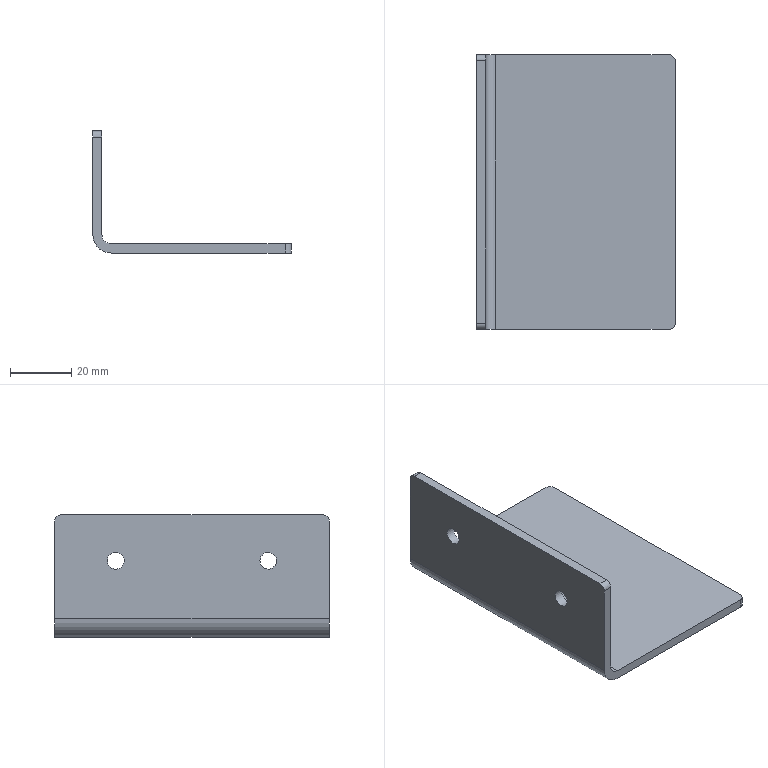Part | NX | features 5003_229_Bracket 2 | 1 solid | 16 faces | box 65 x 90 x 40 mm | volume 26866 mm3 | plane 8 | cylinder 8 | commonest cylinder face diameters 4 x4 5.5 x2 6 x1 12 x1
STEP:
#1=CARTESIAN_POINT('',(218.525,-127.,-84.75));
#2=VERTEX_POINT('',#1);
#3=CARTESIAN_POINT('',(218.525,-127.,-82.));
#4=DIRECTION('',(1.,0.,0.));
#5=DIRECTION('',(0.,0.,-1.));
#6=AXIS2_PLACEMENT_3D('',#3,#4,#5);
#7=CIRCLE('',#6,2.75);
#8=EDGE_CURVE('',#2,#2,#7,.T.);
#9=ORIENTED_EDGE('',*,*,#8,.T.);
#10=EDGE_LOOP('',(#9));
#11=FACE_BOUND('',#10,.T.);
#12=CARTESIAN_POINT('',(218.525,-77.,-84.75));
#13=VERTEX_POINT('',#12);
#14=CARTESIAN_POINT('',(218.525,-77.,-82.));
#15=DIRECTION('',(1.,0.,0.));
#16=DIRECTION('',(0.,0.,-1.));
#17=AXIS2_PLACEMENT_3D('',#14,#15,#16);
#18=CIRCLE('',#17,2.75);
#19=EDGE_CURVE('',#13,#13,#18,.T.);
#20=ORIENTED_EDGE('',*,*,#19,.T.);
#21=EDGE_LOOP('',(#20));
#22=FACE_BOUND('',#21,.T.);
#23=CARTESIAN_POINT('',(218.525,-59.,-67.));
#24=VERTEX_POINT('',#23);
#25=CARTESIAN_POINT('',(218.525,-145.,-67.));
#26=VERTEX_POINT('',#25);
#27=CARTESIAN_POINT('',(218.525,-27.,-67.));
#28=DIRECTION('',(0.,-1.,0.));
#29=VECTOR('',#28,1000.);
#30=LINE('',#27,#29);
#31=EDGE_CURVE('',#24,#26,#30,.T.);
#32=ORIENTED_EDGE('',*,*,#31,.F.);
#33=CARTESIAN_POINT('',(218.525,-57.,-69.));
#34=VERTEX_POINT('',#33);
#35=CARTESIAN_POINT('',(218.525,-59.,-69.));
#36=DIRECTION('',(1.,0.,0.));
#37=DIRECTION('',(0.,0.,-1.));
#38=AXIS2_PLACEMENT_3D('',#35,#36,#37);
#39=CIRCLE('',#38,2.);
#40=EDGE_CURVE('',#24,#34,#39,.F.);
#41=ORIENTED_EDGE('',*,*,#40,.T.);
#42=CARTESIAN_POINT('',(218.525,-57.,-101.));
#43=VERTEX_POINT('',#42);
#44=CARTESIAN_POINT('',(218.525,-57.,-107.));
#45=DIRECTION('',(0.,0.,1.));
#46=VECTOR('',#45,1000.);
#47=LINE('',#44,#46);
#48=EDGE_CURVE('',#43,#34,#47,.T.);
#49=ORIENTED_EDGE('',*,*,#48,.F.);
#50=CARTESIAN_POINT('',(218.525,-147.,-101.));
#51=VERTEX_POINT('',#50);
#52=CARTESIAN_POINT('',(218.525,-27.,-101.));
#53=DIRECTION('',(0.,-1.,0.));
#54=VECTOR('',#53,1000.);
#55=LINE('',#52,#54);
#56=EDGE_CURVE('',#43,#51,#55,.T.);
#57=ORIENTED_EDGE('',*,*,#56,.T.);
#58=CARTESIAN_POINT('',(218.525,-147.,-69.));
#59=VERTEX_POINT('',#58);
#60=CARTESIAN_POINT('',(218.525,-147.,-67.));
#61=DIRECTION('',(0.,0.,1.));
#62=VECTOR('',#61,1000.);
#63=LINE('',#60,#62);
#64=EDGE_CURVE('',#51,#59,#63,.T.);
#65=ORIENTED_EDGE('',*,*,#64,.T.);
#66=CARTESIAN_POINT('',(218.525,-145.,-69.));
#67=DIRECTION('',(1.,0.,0.));
#68=DIRECTION('',(0.,0.,-1.));
#69=AXIS2_PLACEMENT_3D('',#66,#67,#68);
#70=CIRCLE('',#69,2.);
#71=EDGE_CURVE('',#59,#26,#70,.F.);
#72=ORIENTED_EDGE('',*,*,#71,.T.);
#73=EDGE_LOOP('',(#32,#41,#49,#57,#65,#72));
#74=FACE_BOUND('',#73,.T.);
#75=CARTESIAN_POINT('',(218.525,-27.,-67.));
#76=DIRECTION('',(1.,0.,0.));
#77=DIRECTION('',(0.,0.,-1.));
#78=AXIS2_PLACEMENT_3D('',#75,#76,#77);
#79=PLANE('',#78);
#80=ADVANCED_FACE('',(#11,#22,#74),#79,.F.);
#81=CARTESIAN_POINT('',(221.525,-59.,-67.));
#82=VERTEX_POINT('',#81);
#83=CARTESIAN_POINT('',(221.525,-145.,-67.));
#84=VERTEX_POINT('',#83);
#85=CARTESIAN_POINT('',(221.525,-27.,-67.));
#86=DIRECTION('',(0.,-1.,0.));
#87=VECTOR('',#86,1000.);
#88=LINE('',#85,#87);
#89=EDGE_CURVE('',#82,#84,#88,.T.);
#90=ORIENTED_EDGE('',*,*,#89,.F.);
#91=CARTESIAN_POINT('',(221.525,-59.,-67.));
#92=DIRECTION('',(1.,0.,0.));
#93=VECTOR('',#92,1000.);
#94=LINE('',#91,#93);
#95=EDGE_CURVE('',#82,#24,#94,.F.);
#96=ORIENTED_EDGE('',*,*,#95,.T.);
#97=ORIENTED_EDGE('',*,*,#31,.T.);
#98=CARTESIAN_POINT('',(221.525,-145.,-67.));
#99=DIRECTION('',(1.,0.,0.));
#100=VECTOR('',#99,1000.);
#101=LINE('',#98,#100);
#102=EDGE_CURVE('',#26,#84,#101,.T.);
#103=ORIENTED_EDGE('',*,*,#102,.T.);
#104=EDGE_LOOP('',(#90,#96,#97,#103));
#105=FACE_BOUND('',#104,.T.);
#106=CARTESIAN_POINT('',(221.525,-27.,-67.));
#107=DIRECTION('',(0.,0.,-1.));
#108=DIRECTION('',(0.,1.,0.));
#109=AXIS2_PLACEMENT_3D('',#106,#107,#108);
#110=PLANE('',#109);
#111=ADVANCED_FACE('',(#105),#110,.F.);
#112=CARTESIAN_POINT('',(221.525,-124.25,-82.));
#113=VERTEX_POINT('',#112);
#114=CARTESIAN_POINT('',(221.525,-127.,-82.));
#115=DIRECTION('',(1.,0.,0.));
#116=DIRECTION('',(0.,1.,0.));
#117=AXIS2_PLACEMENT_3D('',#114,#115,#116);
#118=CIRCLE('',#117,2.75);
#119=EDGE_CURVE('',#113,#113,#118,.T.);
#120=ORIENTED_EDGE('',*,*,#119,.F.);
#121=EDGE_LOOP('',(#120));
#122=FACE_BOUND('',#121,.T.);
#123=CARTESIAN_POINT('',(221.525,-77.,-79.25));
#124=VERTEX_POINT('',#123);
#125=CARTESIAN_POINT('',(221.525,-77.,-82.));
#126=DIRECTION('',(-1.,0.,0.));
#127=DIRECTION('',(0.,0.,1.));
#128=AXIS2_PLACEMENT_3D('',#125,#126,#127);
#129=CIRCLE('',#128,2.75);
#130=EDGE_CURVE('',#124,#124,#129,.F.);
#131=ORIENTED_EDGE('',*,*,#130,.F.);
#132=EDGE_LOOP('',(#131));
#133=FACE_BOUND('',#132,.T.);
#134=CARTESIAN_POINT('',(221.525,-57.,-69.));
#135=VERTEX_POINT('',#134);
#136=CARTESIAN_POINT('',(221.525,-57.,-101.));
#137=VERTEX_POINT('',#136);
#138=CARTESIAN_POINT('',(221.525,-57.,-107.));
#139=DIRECTION('',(0.,0.,-1.));
#140=VECTOR('',#139,1000.);
#141=LINE('',#138,#140);
#142=EDGE_CURVE('',#135,#137,#141,.T.);
#143=ORIENTED_EDGE('',*,*,#142,.F.);
#144=CARTESIAN_POINT('',(221.525,-59.,-69.));
#145=DIRECTION('',(-1.,0.,0.));
#146=DIRECTION('',(0.,0.,1.));
#147=AXIS2_PLACEMENT_3D('',#144,#145,#146);
#148=CIRCLE('',#147,2.);
#149=EDGE_CURVE('',#135,#82,#148,.F.);
#150=ORIENTED_EDGE('',*,*,#149,.T.);
#151=ORIENTED_EDGE('',*,*,#89,.T.);
#152=CARTESIAN_POINT('',(221.525,-147.,-69.));
#153=VERTEX_POINT('',#152);
#154=CARTESIAN_POINT('',(221.525,-145.,-69.));
#155=DIRECTION('',(-1.,0.,0.));
#156=DIRECTION('',(0.,0.,1.));
#157=AXIS2_PLACEMENT_3D('',#154,#155,#156);
#158=CIRCLE('',#157,2.);
#159=EDGE_CURVE('',#84,#153,#158,.F.);
#160=ORIENTED_EDGE('',*,*,#159,.T.);
#161=CARTESIAN_POINT('',(221.525,-147.,-101.));
#162=VERTEX_POINT('',#161);
#163=CARTESIAN_POINT('',(221.525,-147.,-104.));
#164=DIRECTION('',(0.,0.,-1.));
#165=VECTOR('',#164,1000.);
#166=LINE('',#163,#165);
#167=EDGE_CURVE('',#153,#162,#166,.T.);
#168=ORIENTED_EDGE('',*,*,#167,.T.);
#169=CARTESIAN_POINT('',(221.525,-27.,-101.));
#170=DIRECTION('',(0.,-1.,0.));
#171=VECTOR('',#170,1000.);
#172=LINE('',#169,#171);
#173=EDGE_CURVE('',#162,#137,#172,.F.);
#174=ORIENTED_EDGE('',*,*,#173,.T.);
#175=EDGE_LOOP('',(#143,#150,#151,#160,#168,#174));
#176=FACE_BOUND('',#175,.T.);
#177=CARTESIAN_POINT('',(221.525,-27.,-104.));
#178=DIRECTION('',(-1.,0.,0.));
#179=DIRECTION('',(0.,0.,1.));
#180=AXIS2_PLACEMENT_3D('',#177,#178,#179);
#181=PLANE('',#180);
#182=ADVANCED_FACE('',(#122,#133,#176),#181,.F.);
#183=CARTESIAN_POINT('',(283.525,-59.,-104.));
#184=VERTEX_POINT('',#183);
#185=CARTESIAN_POINT('',(283.525,-145.,-104.));
#186=VERTEX_POINT('',#185);
#187=CARTESIAN_POINT('',(283.525,-27.,-104.));
#188=DIRECTION('',(0.,-1.,0.));
#189=VECTOR('',#188,1000.);
#190=LINE('',#187,#189);
#191=EDGE_CURVE('',#184,#186,#190,.T.);
#192=ORIENTED_EDGE('',*,*,#191,.F.);
#193=CARTESIAN_POINT('',(281.525,-57.,-104.));
#194=VERTEX_POINT('',#193);
#195=CARTESIAN_POINT('',(281.525,-59.,-104.));
#196=DIRECTION('',(0.,0.,-1.));
#197=DIRECTION('',(-1.,0.,0.));
#198=AXIS2_PLACEMENT_3D('',#195,#196,#197);
#199=CIRCLE('',#198,2.);
#200=EDGE_CURVE('',#184,#194,#199,.F.);
#201=ORIENTED_EDGE('',*,*,#200,.T.);
#202=CARTESIAN_POINT('',(224.525,-57.,-104.));
#203=VERTEX_POINT('',#202);
#204=CARTESIAN_POINT('',(283.525,-57.,-104.));
#205=DIRECTION('',(1.,0.,0.));
#206=VECTOR('',#205,1000.);
#207=LINE('',#204,#206);
#208=EDGE_CURVE('',#203,#194,#207,.T.);
#209=ORIENTED_EDGE('',*,*,#208,.F.);
#210=CARTESIAN_POINT('',(224.525,-147.,-104.));
#211=VERTEX_POINT('',#210);
#212=CARTESIAN_POINT('',(224.525,-177.,-104.));
#213=DIRECTION('',(0.,-1.,0.));
#214=VECTOR('',#213,1000.);
#215=LINE('',#212,#214);
#216=EDGE_CURVE('',#203,#211,#215,.T.);
#217=ORIENTED_EDGE('',*,*,#216,.T.);
#218=CARTESIAN_POINT('',(281.525,-147.,-104.));
#219=VERTEX_POINT('',#218);
#220=CARTESIAN_POINT('',(283.525,-147.,-104.));
#221=DIRECTION('',(1.,0.,0.));
#222=VECTOR('',#221,1000.);
#223=LINE('',#220,#222);
#224=EDGE_CURVE('',#211,#219,#223,.T.);
#225=ORIENTED_EDGE('',*,*,#224,.T.);
#226=CARTESIAN_POINT('',(281.525,-145.,-104.));
#227=DIRECTION('',(0.,0.,-1.));
#228=DIRECTION('',(-1.,0.,0.));
#229=AXIS2_PLACEMENT_3D('',#226,#227,#228);
#230=CIRCLE('',#229,2.);
#231=EDGE_CURVE('',#219,#186,#230,.F.);
#232=ORIENTED_EDGE('',*,*,#231,.T.);
#233=EDGE_LOOP('',(#192,#201,#209,#217,#225,#232));
#234=FACE_BOUND('',#233,.T.);
#235=CARTESIAN_POINT('',(283.525,-57.,-104.));
#236=DIRECTION('',(0.,0.,-1.));
#237=DIRECTION('',(-1.,0.,0.));
#238=AXIS2_PLACEMENT_3D('',#235,#236,#237);
#239=PLANE('',#238);
#240=ADVANCED_FACE('',(#234),#239,.F.);
#241=CARTESIAN_POINT('',(283.525,-59.,-107.));
#242=VERTEX_POINT('',#241);
#243=CARTESIAN_POINT('',(283.525,-145.,-107.));
#244=VERTEX_POINT('',#243);
#245=CARTESIAN_POINT('',(283.525,-27.,-107.));
#246=DIRECTION('',(0.,-1.,0.));
#247=VECTOR('',#246,1000.);
#248=LINE('',#245,#247);
#249=EDGE_CURVE('',#242,#244,#248,.T.);
#250=ORIENTED_EDGE('',*,*,#249,.F.);
#251=CARTESIAN_POINT('',(283.525,-59.,-107.));
#252=DIRECTION('',(0.,0.,-1.));
#253=VECTOR('',#252,1000.);
#254=LINE('',#251,#253);
#255=EDGE_CURVE('',#242,#184,#254,.F.);
#256=ORIENTED_EDGE('',*,*,#255,.T.);
#257=ORIENTED_EDGE('',*,*,#191,.T.);
#258=CARTESIAN_POINT('',(283.525,-145.,-107.));
#259=DIRECTION('',(0.,0.,-1.));
#260=VECTOR('',#259,1000.);
#261=LINE('',#258,#260);
#262=EDGE_CURVE('',#186,#244,#261,.T.);
#263=ORIENTED_EDGE('',*,*,#262,.T.);
#264=EDGE_LOOP('',(#250,#256,#257,#263));
#265=FACE_BOUND('',#264,.T.);
#266=CARTESIAN_POINT('',(283.525,-27.,-107.));
#267=DIRECTION('',(-1.,0.,0.));
#268=DIRECTION('',(0.,-1.,0.));
#269=AXIS2_PLACEMENT_3D('',#266,#267,#268);
#270=PLANE('',#269);
#271=ADVANCED_FACE('',(#265),#270,.F.);
#272=CARTESIAN_POINT('',(281.525,-57.,-107.));
#273=VERTEX_POINT('',#272);
#274=CARTESIAN_POINT('',(224.525,-57.,-107.));
#275=VERTEX_POINT('',#274);
#276=CARTESIAN_POINT('',(218.525,-57.,-107.));
#277=DIRECTION('',(-1.,0.,0.));
#278=VECTOR('',#277,1000.);
#279=LINE('',#276,#278);
#280=EDGE_CURVE('',#273,#275,#279,.T.);
#281=ORIENTED_EDGE('',*,*,#280,.F.);
#282=CARTESIAN_POINT('',(281.525,-59.,-107.));
#283=DIRECTION('',(0.,0.,1.));
#284=DIRECTION('',(0.,-1.,0.));
#285=AXIS2_PLACEMENT_3D('',#282,#283,#284);
#286=CIRCLE('',#285,2.);
#287=EDGE_CURVE('',#273,#242,#286,.F.);
#288=ORIENTED_EDGE('',*,*,#287,.T.);
#289=ORIENTED_EDGE('',*,*,#249,.T.);
#290=CARTESIAN_POINT('',(281.525,-147.,-107.));
#291=VERTEX_POINT('',#290);
#292=CARTESIAN_POINT('',(281.525,-145.,-107.));
#293=DIRECTION('',(0.,0.,1.));
#294=DIRECTION('',(0.,-1.,0.));
#295=AXIS2_PLACEMENT_3D('',#292,#293,#294);
#296=CIRCLE('',#295,2.);
#297=EDGE_CURVE('',#244,#291,#296,.F.);
#298=ORIENTED_EDGE('',*,*,#297,.T.);
#299=CARTESIAN_POINT('',(224.525,-147.,-107.));
#300=VERTEX_POINT('',#299);
#301=CARTESIAN_POINT('',(218.525,-147.,-107.));
#302=DIRECTION('',(-1.,0.,0.));
#303=VECTOR('',#302,1000.);
#304=LINE('',#301,#303);
#305=EDGE_CURVE('',#291,#300,#304,.T.);
#306=ORIENTED_EDGE('',*,*,#305,.T.);
#307=CARTESIAN_POINT('',(224.525,-27.,-107.));
#308=DIRECTION('',(0.,-1.,0.));
#309=VECTOR('',#308,1000.);
#310=LINE('',#307,#309);
#311=EDGE_CURVE('',#300,#275,#310,.F.);
#312=ORIENTED_EDGE('',*,*,#311,.T.);
#313=EDGE_LOOP('',(#281,#288,#289,#298,#306,#312));
#314=FACE_BOUND('',#313,.T.);
#315=CARTESIAN_POINT('',(218.525,-27.,-107.));
#316=DIRECTION('',(0.,0.,1.));
#317=DIRECTION('',(0.,-1.,0.));
#318=AXIS2_PLACEMENT_3D('',#315,#316,#317);
#319=PLANE('',#318);
#320=ADVANCED_FACE('',(#314),#319,.F.);
#321=ORIENTED_EDGE('',*,*,#208,.T.);
#322=CARTESIAN_POINT('',(281.525,-57.,-107.));
#323=DIRECTION('',(0.,0.,-1.));
#324=VECTOR('',#323,1000.);
#325=LINE('',#322,#324);
#326=EDGE_CURVE('',#194,#273,#325,.T.);
#327=ORIENTED_EDGE('',*,*,#326,.T.);
#328=ORIENTED_EDGE('',*,*,#280,.T.);
#329=CARTESIAN_POINT('',(224.525,-57.,-101.));
#330=DIRECTION('',(0.,-1.,0.));
#331=DIRECTION('',(0.,0.,-1.));
#332=AXIS2_PLACEMENT_3D('',#329,#330,#331);
#333=CIRCLE('',#332,6.);
#334=EDGE_CURVE('',#275,#43,#333,.F.);
#335=ORIENTED_EDGE('',*,*,#334,.T.);
#336=ORIENTED_EDGE('',*,*,#48,.T.);
#337=CARTESIAN_POINT('',(218.525,-57.,-69.));
#338=DIRECTION('',(1.,0.,0.));
#339=VECTOR('',#338,1000.);
#340=LINE('',#337,#339);
#341=EDGE_CURVE('',#34,#135,#340,.T.);
#342=ORIENTED_EDGE('',*,*,#341,.T.);
#343=ORIENTED_EDGE('',*,*,#142,.T.);
#344=CARTESIAN_POINT('',(224.525,-57.,-101.));
#345=DIRECTION('',(0.,-1.,0.));
#346=DIRECTION('',(0.,0.,-1.));
#347=AXIS2_PLACEMENT_3D('',#344,#345,#346);
#348=CIRCLE('',#347,3.);
#349=EDGE_CURVE('',#137,#203,#348,.T.);
#350=ORIENTED_EDGE('',*,*,#349,.T.);
#351=EDGE_LOOP('',(#321,#327,#328,#335,#336,#342,#343,#350));
#352=FACE_BOUND('',#351,.T.);
#353=CARTESIAN_POINT('',(218.525,-57.,-107.));
#354=DIRECTION('',(0.,-1.,0.));
#355=DIRECTION('',(0.,0.,-1.));
#356=AXIS2_PLACEMENT_3D('',#353,#354,#355);
#357=PLANE('',#356);
#358=ADVANCED_FACE('',(#352),#357,.F.);
#359=ORIENTED_EDGE('',*,*,#305,.F.);
#360=CARTESIAN_POINT('',(281.525,-147.,-104.));
#361=DIRECTION('',(0.,0.,-1.));
#362=VECTOR('',#361,1000.);
#363=LINE('',#360,#362);
#364=EDGE_CURVE('',#291,#219,#363,.F.);
#365=ORIENTED_EDGE('',*,*,#364,.T.);
#366=ORIENTED_EDGE('',*,*,#224,.F.);
#367=CARTESIAN_POINT('',(224.525,-147.,-101.));
#368=DIRECTION('',(0.,-1.,0.));
#369=DIRECTION('',(0.,0.,-1.));
#370=AXIS2_PLACEMENT_3D('',#367,#368,#369);
#371=CIRCLE('',#370,3.);
#372=EDGE_CURVE('',#211,#162,#371,.F.);
#373=ORIENTED_EDGE('',*,*,#372,.T.);
#374=ORIENTED_EDGE('',*,*,#167,.F.);
#375=CARTESIAN_POINT('',(218.525,-147.,-69.));
#376=DIRECTION('',(1.,0.,0.));
#377=VECTOR('',#376,1000.);
#378=LINE('',#375,#377);
#379=EDGE_CURVE('',#153,#59,#378,.F.);
#380=ORIENTED_EDGE('',*,*,#379,.T.);
#381=ORIENTED_EDGE('',*,*,#64,.F.);
#382=CARTESIAN_POINT('',(224.525,-147.,-101.));
#383=DIRECTION('',(0.,-1.,0.));
#384=DIRECTION('',(0.,0.,-1.));
#385=AXIS2_PLACEMENT_3D('',#382,#383,#384);
#386=CIRCLE('',#385,6.);
#387=EDGE_CURVE('',#51,#300,#386,.T.);
#388=ORIENTED_EDGE('',*,*,#387,.T.);
#389=EDGE_LOOP('',(#359,#365,#366,#373,#374,#380,#381,#388));
#390=FACE_BOUND('',#389,.T.);
#391=CARTESIAN_POINT('',(218.525,-147.,-107.));
#392=DIRECTION('',(0.,-1.,0.));
#393=DIRECTION('',(0.,0.,-1.));
#394=AXIS2_PLACEMENT_3D('',#391,#392,#393);
#395=PLANE('',#394);
#396=ADVANCED_FACE('',(#390),#395,.T.);
#397=ORIENTED_EDGE('',*,*,#334,.F.);
#398=ORIENTED_EDGE('',*,*,#311,.F.);
#399=ORIENTED_EDGE('',*,*,#387,.F.);
#400=ORIENTED_EDGE('',*,*,#56,.F.);
#401=EDGE_LOOP('',(#397,#398,#399,#400));
#402=FACE_BOUND('',#401,.T.);
#403=CARTESIAN_POINT('',(224.525,-27.,-101.));
#404=DIRECTION('',(0.,-1.,0.));
#405=DIRECTION('',(0.,0.,-1.));
#406=AXIS2_PLACEMENT_3D('',#403,#404,#405);
#407=CYLINDRICAL_SURFACE('',#406,6.);
#408=ADVANCED_FACE('',(#402),#407,.T.);
#409=ORIENTED_EDGE('',*,*,#349,.F.);
#410=ORIENTED_EDGE('',*,*,#173,.F.);
#411=ORIENTED_EDGE('',*,*,#372,.F.);
#412=ORIENTED_EDGE('',*,*,#216,.F.);
#413=EDGE_LOOP('',(#409,#410,#411,#412));
#414=FACE_BOUND('',#413,.T.);
#415=CARTESIAN_POINT('',(224.525,-57.,-101.));
#416=DIRECTION('',(0.,1.,0.));
#417=DIRECTION('',(0.,0.,1.));
#418=AXIS2_PLACEMENT_3D('',#415,#416,#417);
#419=CYLINDRICAL_SURFACE('',#418,3.);
#420=ADVANCED_FACE('',(#414),#419,.F.);
#421=ORIENTED_EDGE('',*,*,#130,.T.);
#422=EDGE_LOOP('',(#421));
#423=FACE_BOUND('',#422,.T.);
#424=ORIENTED_EDGE('',*,*,#19,.F.);
#425=EDGE_LOOP('',(#424));
#426=FACE_BOUND('',#425,.T.);
#427=CARTESIAN_POINT('',(221.525,-77.,-82.));
#428=DIRECTION('',(1.,0.,0.));
#429=DIRECTION('',(0.,1.,0.));
#430=AXIS2_PLACEMENT_3D('',#427,#428,#429);
#431=CYLINDRICAL_SURFACE('',#430,2.75);
#432=ADVANCED_FACE('',(#423,#426),#431,.F.);
#433=ORIENTED_EDGE('',*,*,#119,.T.);
#434=EDGE_LOOP('',(#433));
#435=FACE_BOUND('',#434,.T.);
#436=ORIENTED_EDGE('',*,*,#8,.F.);
#437=EDGE_LOOP('',(#436));
#438=FACE_BOUND('',#437,.T.);
#439=CARTESIAN_POINT('',(221.525,-127.,-82.));
#440=DIRECTION('',(1.,0.,0.));
#441=DIRECTION('',(0.,1.,0.));
#442=AXIS2_PLACEMENT_3D('',#439,#440,#441);
#443=CYLINDRICAL_SURFACE('',#442,2.75);
#444=ADVANCED_FACE('',(#435,#438),#443,.F.);
#445=ORIENTED_EDGE('',*,*,#200,.F.);
#446=ORIENTED_EDGE('',*,*,#255,.F.);
#447=ORIENTED_EDGE('',*,*,#287,.F.);
#448=ORIENTED_EDGE('',*,*,#326,.F.);
#449=EDGE_LOOP('',(#445,#446,#447,#448));
#450=FACE_BOUND('',#449,.T.);
#451=CARTESIAN_POINT('',(281.525,-59.,-107.));
#452=DIRECTION('',(0.,0.,-1.));
#453=DIRECTION('',(0.,1.,0.));
#454=AXIS2_PLACEMENT_3D('',#451,#452,#453);
#455=CYLINDRICAL_SURFACE('',#454,2.);
#456=ADVANCED_FACE('',(#450),#455,.T.);
#457=ORIENTED_EDGE('',*,*,#231,.F.);
#458=ORIENTED_EDGE('',*,*,#364,.F.);
#459=ORIENTED_EDGE('',*,*,#297,.F.);
#460=ORIENTED_EDGE('',*,*,#262,.F.);
#461=EDGE_LOOP('',(#457,#458,#459,#460));
#462=FACE_BOUND('',#461,.T.);
#463=CARTESIAN_POINT('',(281.525,-145.,-107.));
#464=DIRECTION('',(0.,0.,1.));
#465=DIRECTION('',(0.,-1.,0.));
#466=AXIS2_PLACEMENT_3D('',#463,#464,#465);
#467=CYLINDRICAL_SURFACE('',#466,2.);
#468=ADVANCED_FACE('',(#462),#467,.T.);
#469=ORIENTED_EDGE('',*,*,#40,.F.);
#470=ORIENTED_EDGE('',*,*,#95,.F.);
#471=ORIENTED_EDGE('',*,*,#149,.F.);
#472=ORIENTED_EDGE('',*,*,#341,.F.);
#473=EDGE_LOOP('',(#469,#470,#471,#472));
#474=FACE_BOUND('',#473,.T.);
#475=CARTESIAN_POINT('',(218.525,-59.,-69.));
#476=DIRECTION('',(1.,0.,0.));
#477=DIRECTION('',(0.,1.,0.));
#478=AXIS2_PLACEMENT_3D('',#475,#476,#477);
#479=CYLINDRICAL_SURFACE('',#478,2.);
#480=ADVANCED_FACE('',(#474),#479,.T.);
#481=ORIENTED_EDGE('',*,*,#71,.F.);
#482=ORIENTED_EDGE('',*,*,#379,.F.);
#483=ORIENTED_EDGE('',*,*,#159,.F.);
#484=ORIENTED_EDGE('',*,*,#102,.F.);
#485=EDGE_LOOP('',(#481,#482,#483,#484));
#486=FACE_BOUND('',#485,.T.);
#487=CARTESIAN_POINT('',(221.525,-145.,-69.));
#488=DIRECTION('',(-1.,0.,0.));
#489=DIRECTION('',(0.,-1.,0.));
#490=AXIS2_PLACEMENT_3D('',#487,#488,#489);
#491=CYLINDRICAL_SURFACE('',#490,2.);
#492=ADVANCED_FACE('',(#486),#491,.T.);
#493=CLOSED_SHELL('',(#80,#111,#182,#240,#271,#320,#358,#396,#408,#420,#432,#444,#456,#468,#480,#492));
#494=MANIFOLD_SOLID_BREP('',#493);
#495=(LENGTH_UNIT()NAMED_UNIT(*)SI_UNIT(.MILLI.,.METRE.));
#496=UNCERTAINTY_MEASURE_WITH_UNIT(LENGTH_MEASURE(0.00001),#495,'','');
#497=(NAMED_UNIT(*)PLANE_ANGLE_UNIT()SI_UNIT($,.RADIAN.));
#498=(NAMED_UNIT(*)SI_UNIT($,.STERADIAN.)SOLID_ANGLE_UNIT());
#499=(GEOMETRIC_REPRESENTATION_CONTEXT(3)GLOBAL_UNCERTAINTY_ASSIGNED_CONTEXT((#496))GLOBAL_UNIT_ASSIGNED_CONTEXT((#495,#497,#498))REPRESENTATION_CONTEXT('',''));
#500=ADVANCED_BREP_SHAPE_REPRESENTATION('',(#494),#499);